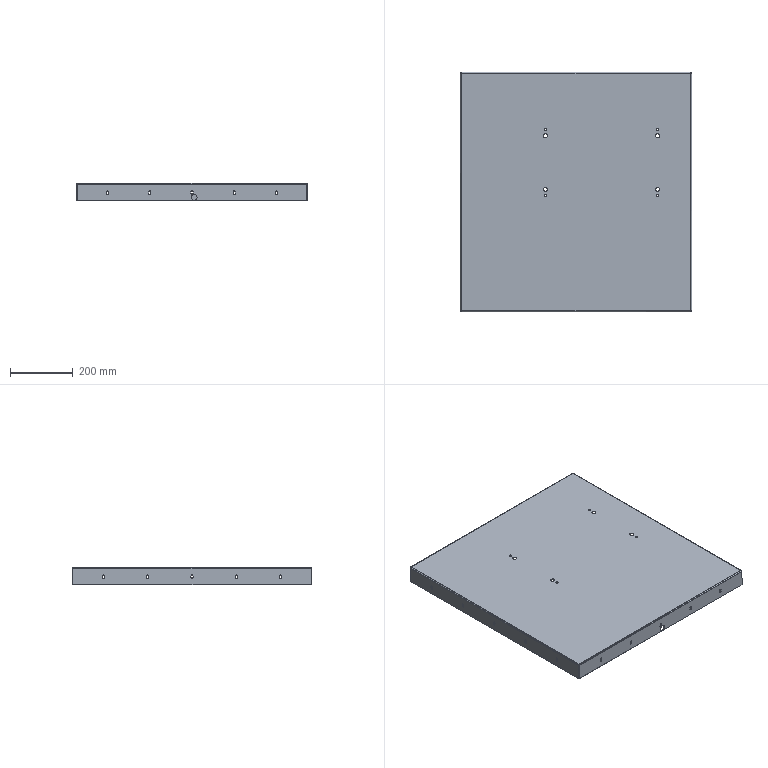Part | STEP file | JBJ-P-1006-05 | 1 solid | 127 faces | box 735 x 762 x 55 mm | volume 1423016 mm3 | plane 62 | cylinder 57 | spline 8 | commonest cylinder face diameters 6.5 x40 4 x4 7.2 x4 8 x4 12.5 x4 18 x1